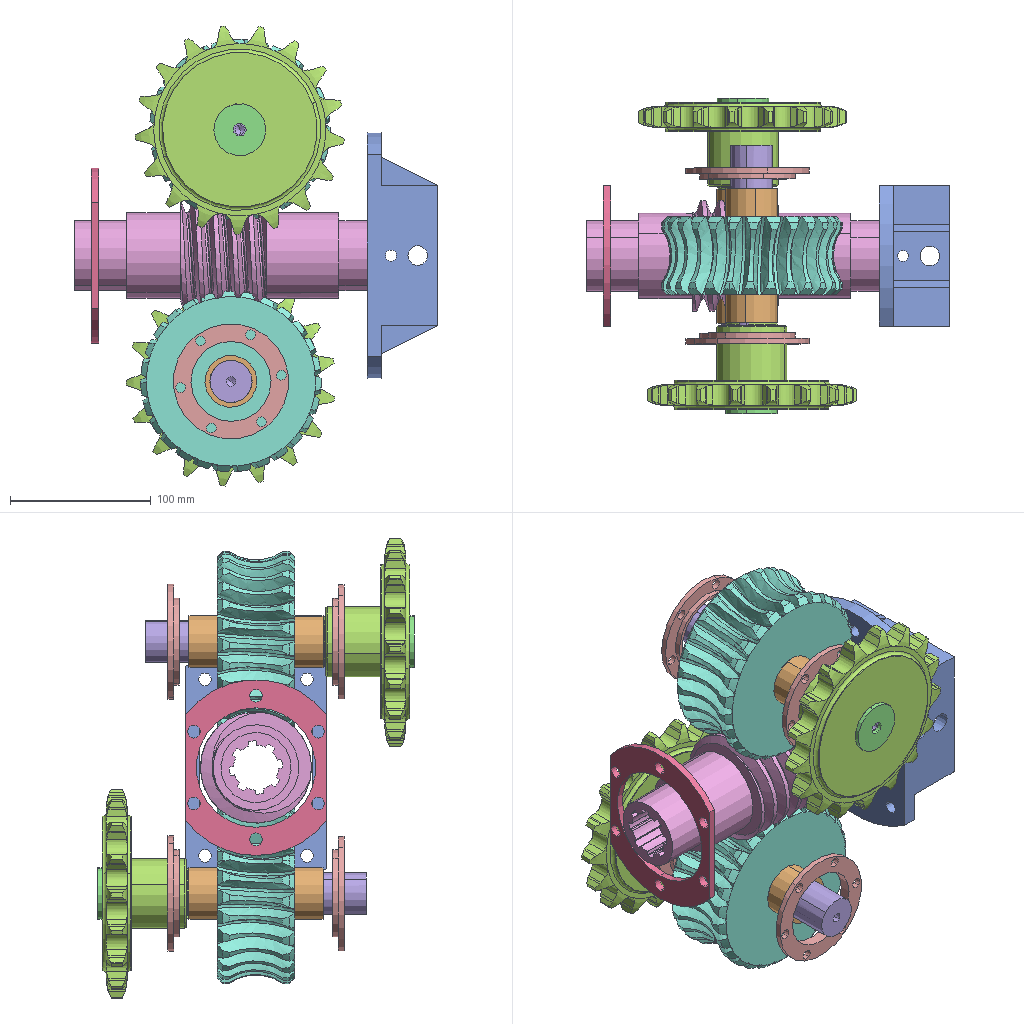Assembly | SolidWorks | 12 different items | 22 placed | box 258 x 225 x 327 mm
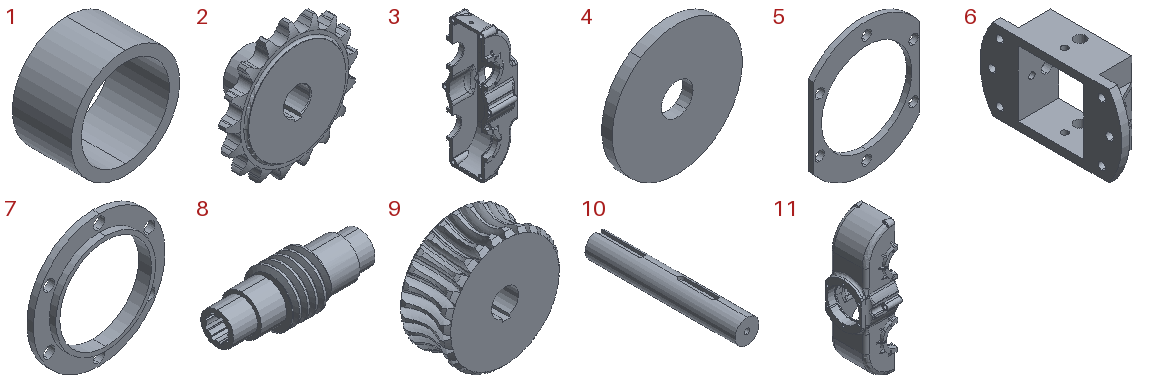Parts list (item | name | quantity | size | volume | features):
1 | - | x4 | 37 x 20 x 37 mm | 7367 mm3 | features BaseBody 1
2 | - | x2 | 148.61 x 61.823 x 148.247 mm | 292316 mm3 | features BaseBody 1
3 | - | x1 | 95.5 x 143.009 x 375 mm | 902272 mm3 | features BaseBody 1, ICE 1
4 | - | x2 | 37 x 3 x 37 mm | 3035 mm3 | features BaseBody 1
5 | - | x1 | 100 x 5 x 125 mm | 24691 mm3 | features ICE 2, Extrusion 1
6 | - | x1 | 50 x 175 x 100 mm | 233318 mm3 | features HoleWzd 4, ICE 4, MirrorPattern 2, Extrusion 1, Rib 1
7 | - | x4 | 82 x 8 x 82 mm | 11863 mm3 | features HoleWzd 2, ICE 1, Revolution 1
8 | - | x1 | 216.6 x 79 x 79 mm | 426843 mm3 | features BaseBody 1
9 | - | x2 | 128.363 x 55.3 x 128.358 mm | 529426 mm3 | features BaseBody 1
10 | - | x2 | 30 x 188 x 30 mm | 126976 mm3 | features BaseBody 1
11 | - | x1 | 95.5 x 143.009 x 375 mm | 821639 mm3 | features BaseBody 3
12 | deep groove ball bearings gb | x1 | - | - | -
Mates (type | each side: item.copy, entity, surface, feature):
Concentric | 2.1 face cylinder | 4.1 face cylinder
Coincident | 2.1 face plane | 4.1 face plane
Coincident | 2.1 face plane | 1.1 face plane
Coincident | 9.1 face plane | 1.1 face plane
Concentric | 2.1 face cylinder | 1.2 face cylinder
Coincident | 9.1 face plane | 1.2 face plane
Symmetric | 8.1 face plane | 8.1 face plane | assembly plane
Concentric | 10.1 face cylinder | 2.2 face cylinder
Coincident | 2.2 face plane | 4.2 face plane
Concentric | 2.2 face cylinder | 4.2 face cylinder
Coincident | 10.1 face plane | 4.2 face plane
Concentric | 10.1 face cylinder | 9.2 face cylinder
Concentric | 10.1 face cylinder | 1.3 face cylinder
Coincident | 9.2 face plane | 1.3 face plane
Coincident | 2.2 face plane | 1.3 face plane
Concentric | 10.1 face cylinder | 1.4 face cylinder
Coincident | 9.2 face plane | 1.4 face plane
Coincident | 9.1 face plane | 9.2 face plane
Concentric | 10.1 face cylinder | 7.1 face cylinder M52 Clearance Hole1
Concentric | 9.1 face cylinder | 10.2 face cylinder
Parallel | 9.1 face plane | 10.2 face plane
Concentric | 9.1 face cylinder | 1.1 face cylinder
Concentric | 10.2 face cylinder | 7.2 face cylinder M52 Clearance Hole1
Concentric | 10.2 face cylinder | 1.2 face cylinder
Coincident | 2.1 face plane | 10.2 face plane
Parallel | 2.1 face plane | 10.2 face plane